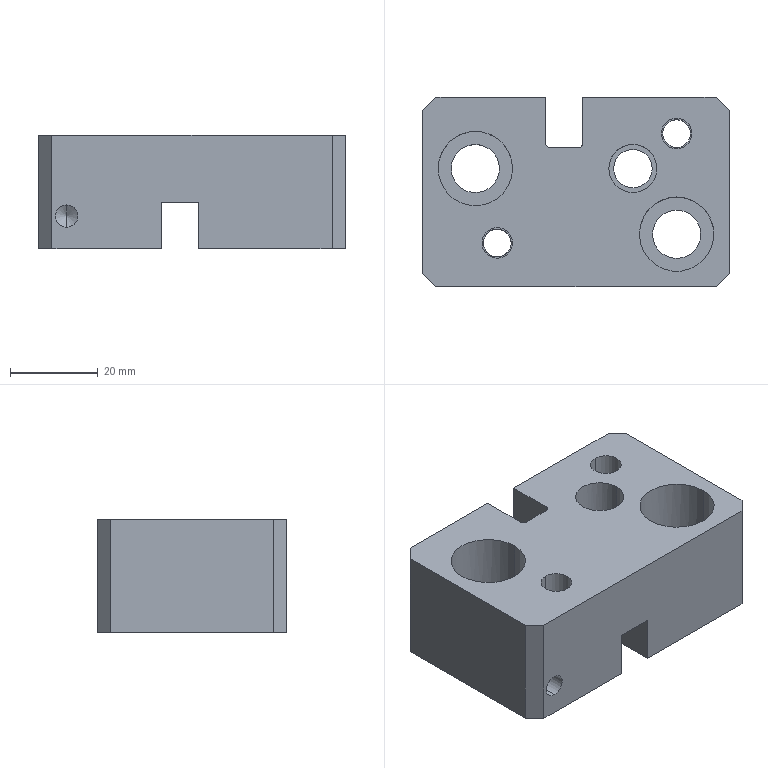Part | STEP file | 1_id994_x_t | 1 solid | 47 faces | box 70 x 43.296 x 26 mm | volume 59877 mm3 | cylinder 24 | plane 21 | cone 2 | commonest cylinder face diameters 11 x6 6.35 x4 7 x4 17 x4 2 x2 5.105 x2